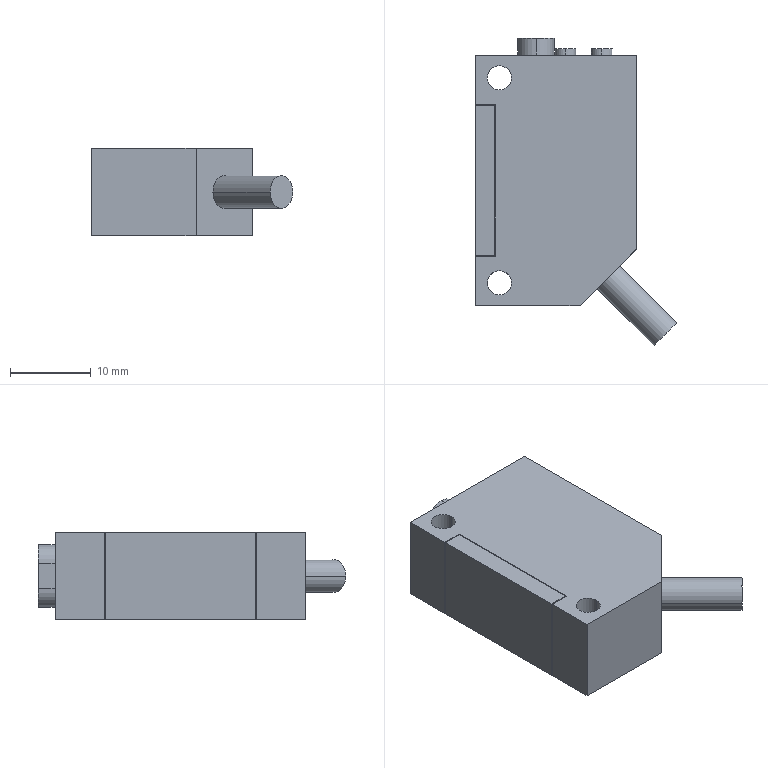Part | STEP file | E3Z-R61 5M_PART1 | 1 solid | 55 faces | box 24.985 x 38.085 x 10.8 mm | volume 6468 mm3 | plane 33 | cylinder 22 | commonest cylinder face diameters 2.6 x4 2.9 x4 3 x4 3.1 x4 4.5 x4 4 x2